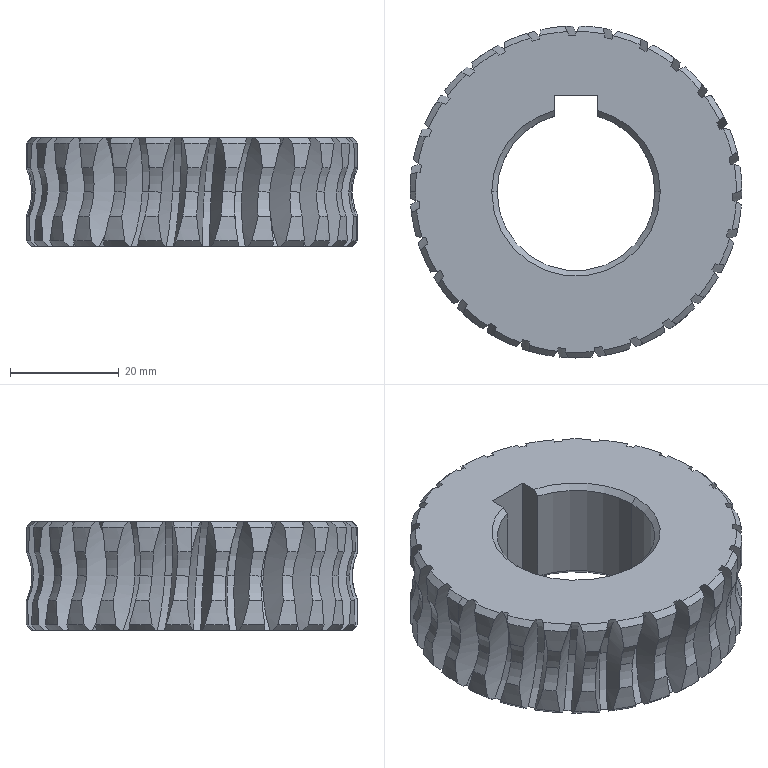Part | SolidWorks | features Chamfer 2, ICE 2, CirPattern 1, Extrusion 1, Helix 1, RevCut 1, SweepCut 1 | 1 solid | 286 faces | box 61 x 60.994 x 20 mm | volume 37460 mm3 | cylinder 111 | cone 62 | torus 54 | spline 54 | plane 5 | commonest cylinder face diameters 61 x55 30 x53 29 x3